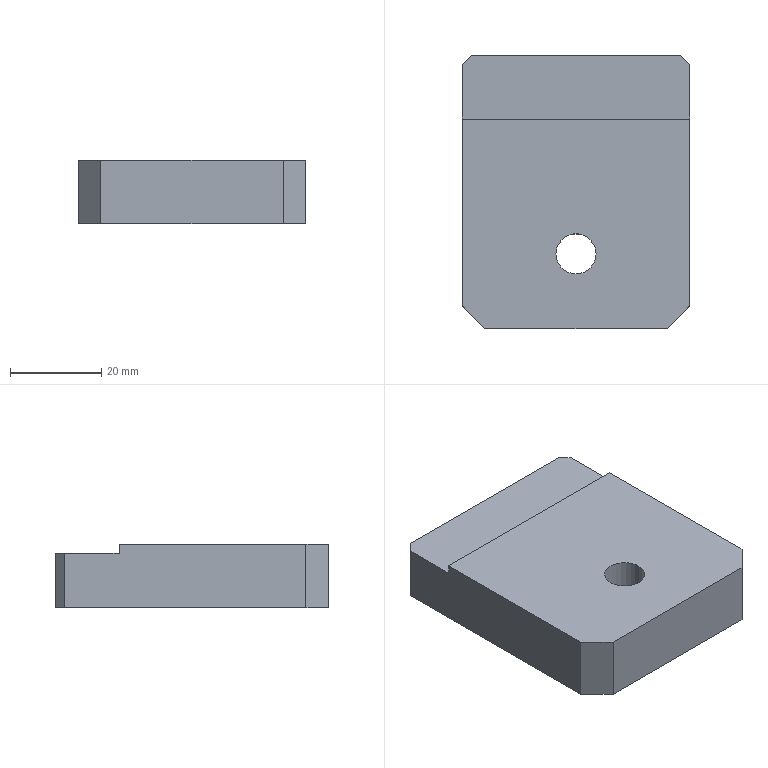Part | STEP file | 2012-06-08-03 | 1 solid | 14 faces | box 50 x 60 x 14 mm | volume 39351 mm3 | plane 12 | cylinder 2 | commonest cylinder face diameters 8.8 x2
STEP:
#1=CARTESIAN_POINT('',(0.,0.,0.));
#2=DIRECTION('',(0.,0.,1.));
#3=DIRECTION('',(1.,0.,0.));
#4=AXIS2_PLACEMENT_3D('',#1,#2,#3);
#5=CARTESIAN_POINT('',(-4.4,-13.59,14.));
#6=VERTEX_POINT('',#5);
#7=CARTESIAN_POINT('',(-4.4,-13.59,0.));
#8=VERTEX_POINT('',#7);
#9=CARTESIAN_POINT('',(-4.4,-13.59,0.));
#10=DIRECTION('',(0.,0.,-1.));
#11=VECTOR('',#10,1.);
#12=LINE('',#9,#11);
#13=CARTESIAN_POINT('',(0.,-13.59,0.));
#14=DIRECTION('',(0.,0.,-1.));
#15=DIRECTION('',(-1.,0.,0.));
#16=AXIS2_PLACEMENT_3D('',#13,#14,#15);
#17=CYLINDRICAL_SURFACE('',#16,4.4);
#18=CARTESIAN_POINT('',(6.283,0.));
#19=DIRECTION('',(0.,1.));
#20=VECTOR('',#19,1.);
#21=LINE('',#18,#20);
#22=(GEOMETRIC_REPRESENTATION_CONTEXT(2)PARAMETRIC_REPRESENTATION_CONTEXT()REPRESENTATION_CONTEXT('',''));
#23=DEFINITIONAL_REPRESENTATION('',(#21),#22);
#24=PCURVE('',#17,#23);
#25=CARTESIAN_POINT('',(0.,-13.59,0.));
#26=DIRECTION('',(0.,0.,-1.));
#27=DIRECTION('',(-1.,0.,0.));
#28=AXIS2_PLACEMENT_3D('',#25,#26,#27);
#29=CYLINDRICAL_SURFACE('',#28,4.4);
#30=CARTESIAN_POINT('',(0.,0.));
#31=DIRECTION('',(0.,1.));
#32=VECTOR('',#31,1.);
#33=LINE('',#30,#32);
#34=(GEOMETRIC_REPRESENTATION_CONTEXT(2)PARAMETRIC_REPRESENTATION_CONTEXT()REPRESENTATION_CONTEXT('',''));
#35=DEFINITIONAL_REPRESENTATION('',(#33),#34);
#36=PCURVE('',#29,#35);
#37=SURFACE_CURVE('',#12,(#24,#36),.PCURVE_S1.);
#38=EDGE_CURVE('',#6,#8,#37,.T.);
#39=ORIENTED_EDGE('',*,*,#38,.T.);
#40=CARTESIAN_POINT('',(4.4,-13.59,0.));
#41=VERTEX_POINT('',#40);
#42=CARTESIAN_POINT('',(0.,-13.59,0.));
#43=DIRECTION('',(0.,0.,-1.));
#44=DIRECTION('',(-1.,0.,0.));
#45=AXIS2_PLACEMENT_3D('',#42,#43,#44);
#46=CIRCLE('',#45,4.4);
#47=CARTESIAN_POINT('',(0.,0.));
#48=DIRECTION('',(1.,0.));
#49=VECTOR('',#48,1.);
#50=LINE('',#47,#49);
#51=(GEOMETRIC_REPRESENTATION_CONTEXT(2)PARAMETRIC_REPRESENTATION_CONTEXT()REPRESENTATION_CONTEXT('',''));
#52=DEFINITIONAL_REPRESENTATION('',(#50),#51);
#53=PCURVE('',#17,#52);
#54=CARTESIAN_POINT('',(25.,-30.,0.));
#55=DIRECTION('',(0.,0.,1.));
#56=DIRECTION('',(1.,0.,0.));
#57=AXIS2_PLACEMENT_3D('',#54,#55,#56);
#58=PLANE('',#57);
#59=CARTESIAN_POINT('',(-29.4,16.41));
#60=CARTESIAN_POINT('',(-29.4,24.031));
#61=CARTESIAN_POINT('',(-22.8,20.221));
#62=CARTESIAN_POINT('',(-16.2,16.41));
#63=CARTESIAN_POINT('',(-22.8,12.599));
#64=CARTESIAN_POINT('',(-29.4,8.789));
#65=CARTESIAN_POINT('',(-29.4,16.41));
#66=(BOUNDED_CURVE()B_SPLINE_CURVE(2,(#59,#60,#61,#62,#63,#64,#65),.UNSPECIFIED.,.T.,.F.)B_SPLINE_CURVE_WITH_KNOTS((1,2,2,2,2,1),(-2.094,0.,2.094,4.189,6.283,8.378),.UNSPECIFIED.)CURVE()GEOMETRIC_REPRESENTATION_ITEM()RATIONAL_B_SPLINE_CURVE((1.,0.5,1.,0.5,1.,0.5,1.))REPRESENTATION_ITEM(''));
#67=(GEOMETRIC_REPRESENTATION_CONTEXT(2)PARAMETRIC_REPRESENTATION_CONTEXT()REPRESENTATION_CONTEXT('',''));
#68=DEFINITIONAL_REPRESENTATION('',(#66),#67);
#69=PCURVE('',#58,#68);
#70=SURFACE_CURVE('',#46,(#53,#69),.PCURVE_S1.);
#71=EDGE_CURVE('',#41,#8,#70,.T.);
#72=ORIENTED_EDGE('',*,*,#71,.F.);
#73=CARTESIAN_POINT('',(4.4,-13.59,14.));
#74=VERTEX_POINT('',#73);
#75=CARTESIAN_POINT('',(4.4,-13.59,0.));
#76=DIRECTION('',(0.,0.,-1.));
#77=VECTOR('',#76,1.);
#78=LINE('',#75,#77);
#79=CARTESIAN_POINT('',(3.142,0.));
#80=DIRECTION('',(0.,1.));
#81=VECTOR('',#80,1.);
#82=LINE('',#79,#81);
#83=(GEOMETRIC_REPRESENTATION_CONTEXT(2)PARAMETRIC_REPRESENTATION_CONTEXT()REPRESENTATION_CONTEXT('',''));
#84=DEFINITIONAL_REPRESENTATION('',(#82),#83);
#85=PCURVE('',#17,#84);
#86=CARTESIAN_POINT('',(3.142,0.));
#87=DIRECTION('',(0.,1.));
#88=VECTOR('',#87,1.);
#89=LINE('',#86,#88);
#90=(GEOMETRIC_REPRESENTATION_CONTEXT(2)PARAMETRIC_REPRESENTATION_CONTEXT()REPRESENTATION_CONTEXT('',''));
#91=DEFINITIONAL_REPRESENTATION('',(#89),#90);
#92=PCURVE('',#29,#91);
#93=SURFACE_CURVE('',#78,(#85,#92),.PCURVE_S1.);
#94=EDGE_CURVE('',#74,#41,#93,.T.);
#95=ORIENTED_EDGE('',*,*,#94,.F.);
#96=CARTESIAN_POINT('',(0.,-13.59,14.));
#97=DIRECTION('',(0.,0.,1.));
#98=DIRECTION('',(1.,0.,0.));
#99=AXIS2_PLACEMENT_3D('',#96,#97,#98);
#100=CIRCLE('',#99,4.4);
#101=CARTESIAN_POINT('',(9.425,-14.));
#102=DIRECTION('',(-1.,0.));
#103=VECTOR('',#102,1.);
#104=LINE('',#101,#103);
#105=(GEOMETRIC_REPRESENTATION_CONTEXT(2)PARAMETRIC_REPRESENTATION_CONTEXT()REPRESENTATION_CONTEXT('',''));
#106=DEFINITIONAL_REPRESENTATION('',(#104),#105);
#107=PCURVE('',#17,#106);
#108=CARTESIAN_POINT('',(25.,-30.,14.));
#109=DIRECTION('',(0.,0.,1.));
#110=DIRECTION('',(1.,0.,0.));
#111=AXIS2_PLACEMENT_3D('',#108,#109,#110);
#112=PLANE('',#111);
#113=CARTESIAN_POINT('',(-25.,16.41));
#114=DIRECTION('',(1.,0.));
#115=AXIS2_PLACEMENT_2D('',#113,#114);
#116=CIRCLE('',#115,4.4);
#117=(GEOMETRIC_REPRESENTATION_CONTEXT(2)PARAMETRIC_REPRESENTATION_CONTEXT()REPRESENTATION_CONTEXT('',''));
#118=DEFINITIONAL_REPRESENTATION('',(#116),#117);
#119=PCURVE('',#112,#118);
#120=SURFACE_CURVE('',#100,(#107,#119),.PCURVE_S1.);
#121=EDGE_CURVE('',#6,#74,#120,.T.);
#122=ORIENTED_EDGE('',*,*,#121,.F.);
#123=EDGE_LOOP('',(#39,#72,#95,#122));
#124=FACE_BOUND('',#123,.F.);
#125=ADVANCED_FACE('',(#124),#17,.F.);
#126=CARTESIAN_POINT('',(23.,30.,12.));
#127=VERTEX_POINT('',#126);
#128=CARTESIAN_POINT('',(-23.,30.,12.));
#129=VERTEX_POINT('',#128);
#130=CARTESIAN_POINT('',(-25.,30.,12.));
#131=DIRECTION('',(-1.,0.,0.));
#132=VECTOR('',#131,1.);
#133=LINE('',#130,#132);
#134=CARTESIAN_POINT('',(-25.,30.,14.));
#135=DIRECTION('',(0.,-1.,0.));
#136=DIRECTION('',(0.,0.,-1.));
#137=AXIS2_PLACEMENT_3D('',#134,#135,#136);
#138=PLANE('',#137);
#139=CARTESIAN_POINT('',(2.,0.));
#140=DIRECTION('',(0.,-1.));
#141=VECTOR('',#140,1.);
#142=LINE('',#139,#141);
#143=(GEOMETRIC_REPRESENTATION_CONTEXT(2)PARAMETRIC_REPRESENTATION_CONTEXT()REPRESENTATION_CONTEXT('',''));
#144=DEFINITIONAL_REPRESENTATION('',(#142),#143);
#145=PCURVE('',#138,#144);
#146=CARTESIAN_POINT('',(-25.,16.,12.));
#147=DIRECTION('',(0.,0.,1.));
#148=DIRECTION('',(1.,0.,0.));
#149=AXIS2_PLACEMENT_3D('',#146,#147,#148);
#150=PLANE('',#149);
#151=CARTESIAN_POINT('',(0.,14.));
#152=DIRECTION('',(-1.,0.));
#153=VECTOR('',#152,1.);
#154=LINE('',#151,#153);
#155=(GEOMETRIC_REPRESENTATION_CONTEXT(2)PARAMETRIC_REPRESENTATION_CONTEXT()REPRESENTATION_CONTEXT('',''));
#156=DEFINITIONAL_REPRESENTATION('',(#154),#155);
#157=PCURVE('',#150,#156);
#158=SURFACE_CURVE('',#133,(#145,#157),.PCURVE_S1.);
#159=EDGE_CURVE('',#127,#129,#158,.T.);
#160=ORIENTED_EDGE('',*,*,#159,.F.);
#161=CARTESIAN_POINT('',(23.,30.,0.));
#162=VERTEX_POINT('',#161);
#163=CARTESIAN_POINT('',(23.,30.,14.));
#164=DIRECTION('',(0.,0.,-1.));
#165=VECTOR('',#164,1.);
#166=LINE('',#163,#165);
#167=CARTESIAN_POINT('',(0.,48.));
#168=DIRECTION('',(1.,0.));
#169=VECTOR('',#168,1.);
#170=LINE('',#167,#169);
#171=(GEOMETRIC_REPRESENTATION_CONTEXT(2)PARAMETRIC_REPRESENTATION_CONTEXT()REPRESENTATION_CONTEXT('',''));
#172=DEFINITIONAL_REPRESENTATION('',(#170),#171);
#173=PCURVE('',#138,#172);
#174=CARTESIAN_POINT('',(23.,30.,14.));
#175=DIRECTION('',(-0.7071,-0.7071,0.));
#176=DIRECTION('',(0.7071,-0.7071,0.));
#177=AXIS2_PLACEMENT_3D('',#174,#175,#176);
#178=PLANE('',#177);
#179=CARTESIAN_POINT('',(0.,0.));
#180=DIRECTION('',(0.,-1.));
#181=VECTOR('',#180,1.);
#182=LINE('',#179,#181);
#183=(GEOMETRIC_REPRESENTATION_CONTEXT(2)PARAMETRIC_REPRESENTATION_CONTEXT()REPRESENTATION_CONTEXT('',''));
#184=DEFINITIONAL_REPRESENTATION('',(#182),#183);
#185=PCURVE('',#178,#184);
#186=SURFACE_CURVE('',#166,(#173,#185),.PCURVE_S1.);
#187=EDGE_CURVE('',#127,#162,#186,.T.);
#188=ORIENTED_EDGE('',*,*,#187,.T.);
#189=CARTESIAN_POINT('',(-23.,30.,0.));
#190=VERTEX_POINT('',#189);
#191=CARTESIAN_POINT('',(-25.,30.,0.));
#192=DIRECTION('',(-1.,0.,0.));
#193=VECTOR('',#192,1.);
#194=LINE('',#191,#193);
#195=CARTESIAN_POINT('',(14.,0.));
#196=DIRECTION('',(0.,-1.));
#197=VECTOR('',#196,1.);
#198=LINE('',#195,#197);
#199=(GEOMETRIC_REPRESENTATION_CONTEXT(2)PARAMETRIC_REPRESENTATION_CONTEXT()REPRESENTATION_CONTEXT('',''));
#200=DEFINITIONAL_REPRESENTATION('',(#198),#199);
#201=PCURVE('',#138,#200);
#202=CARTESIAN_POINT('',(-50.,60.));
#203=DIRECTION('',(-1.,0.));
#204=VECTOR('',#203,1.);
#205=LINE('',#202,#204);
#206=(GEOMETRIC_REPRESENTATION_CONTEXT(2)PARAMETRIC_REPRESENTATION_CONTEXT()REPRESENTATION_CONTEXT('',''));
#207=DEFINITIONAL_REPRESENTATION('',(#205),#206);
#208=PCURVE('',#58,#207);
#209=SURFACE_CURVE('',#194,(#201,#208),.PCURVE_S1.);
#210=EDGE_CURVE('',#162,#190,#209,.T.);
#211=ORIENTED_EDGE('',*,*,#210,.T.);
#212=CARTESIAN_POINT('',(-23.,30.,14.));
#213=DIRECTION('',(0.,0.,1.));
#214=VECTOR('',#213,1.);
#215=LINE('',#212,#214);
#216=CARTESIAN_POINT('',(0.,2.));
#217=DIRECTION('',(-1.,0.));
#218=VECTOR('',#217,1.);
#219=LINE('',#216,#218);
#220=(GEOMETRIC_REPRESENTATION_CONTEXT(2)PARAMETRIC_REPRESENTATION_CONTEXT()REPRESENTATION_CONTEXT('',''));
#221=DEFINITIONAL_REPRESENTATION('',(#219),#220);
#222=PCURVE('',#138,#221);
#223=CARTESIAN_POINT('',(-25.,28.,14.));
#224=DIRECTION('',(0.7071,-0.7071,0.));
#225=DIRECTION('',(0.7071,0.7071,0.));
#226=AXIS2_PLACEMENT_3D('',#223,#224,#225);
#227=PLANE('',#226);
#228=CARTESIAN_POINT('',(2.828,0.));
#229=DIRECTION('',(0.,1.));
#230=VECTOR('',#229,1.);
#231=LINE('',#228,#230);
#232=(GEOMETRIC_REPRESENTATION_CONTEXT(2)PARAMETRIC_REPRESENTATION_CONTEXT()REPRESENTATION_CONTEXT('',''));
#233=DEFINITIONAL_REPRESENTATION('',(#231),#232);
#234=PCURVE('',#227,#233);
#235=SURFACE_CURVE('',#215,(#222,#234),.PCURVE_S1.);
#236=EDGE_CURVE('',#190,#129,#235,.T.);
#237=ORIENTED_EDGE('',*,*,#236,.T.);
#238=EDGE_LOOP('',(#160,#188,#211,#237));
#239=FACE_BOUND('',#238,.T.);
#240=ADVANCED_FACE('',(#239),#138,.F.);
#241=CARTESIAN_POINT('',(25.,-25.,0.));
#242=VERTEX_POINT('',#241);
#243=CARTESIAN_POINT('',(25.,28.,0.));
#244=VERTEX_POINT('',#243);
#245=CARTESIAN_POINT('',(25.,30.,0.));
#246=DIRECTION('',(0.,1.,0.));
#247=VECTOR('',#246,1.);
#248=LINE('',#245,#247);
#249=CARTESIAN_POINT('',(25.,30.,14.));
#250=DIRECTION('',(-1.,0.,0.));
#251=DIRECTION('',(0.,-1.,0.));
#252=AXIS2_PLACEMENT_3D('',#249,#250,#251);
#253=PLANE('',#252);
#254=CARTESIAN_POINT('',(0.,-14.));
#255=DIRECTION('',(-1.,0.));
#256=VECTOR('',#255,1.);
#257=LINE('',#254,#256);
#258=(GEOMETRIC_REPRESENTATION_CONTEXT(2)PARAMETRIC_REPRESENTATION_CONTEXT()REPRESENTATION_CONTEXT('',''));
#259=DEFINITIONAL_REPRESENTATION('',(#257),#258);
#260=PCURVE('',#253,#259);
#261=CARTESIAN_POINT('',(0.,60.));
#262=DIRECTION('',(0.,1.));
#263=VECTOR('',#262,1.);
#264=LINE('',#261,#263);
#265=(GEOMETRIC_REPRESENTATION_CONTEXT(2)PARAMETRIC_REPRESENTATION_CONTEXT()REPRESENTATION_CONTEXT('',''));
#266=DEFINITIONAL_REPRESENTATION('',(#264),#265);
#267=PCURVE('',#58,#266);
#268=SURFACE_CURVE('',#248,(#260,#267),.PCURVE_S1.);
#269=EDGE_CURVE('',#242,#244,#268,.T.);
#270=ORIENTED_EDGE('',*,*,#269,.T.);
#271=CARTESIAN_POINT('',(25.,28.,12.));
#272=VERTEX_POINT('',#271);
#273=CARTESIAN_POINT('',(25.,28.,14.));
#274=DIRECTION('',(0.,0.,1.));
#275=VECTOR('',#274,1.);
#276=LINE('',#273,#275);
#277=CARTESIAN_POINT('',(2.,0.));
#278=DIRECTION('',(0.,1.));
#279=VECTOR('',#278,1.);
#280=LINE('',#277,#279);
#281=(GEOMETRIC_REPRESENTATION_CONTEXT(2)PARAMETRIC_REPRESENTATION_CONTEXT()REPRESENTATION_CONTEXT('',''));
#282=DEFINITIONAL_REPRESENTATION('',(#280),#281);
#283=PCURVE('',#253,#282);
#284=CARTESIAN_POINT('',(2.828,0.));
#285=DIRECTION('',(0.,1.));
#286=VECTOR('',#285,1.);
#287=LINE('',#284,#286);
#288=(GEOMETRIC_REPRESENTATION_CONTEXT(2)PARAMETRIC_REPRESENTATION_CONTEXT()REPRESENTATION_CONTEXT('',''));
#289=DEFINITIONAL_REPRESENTATION('',(#287),#288);
#290=PCURVE('',#178,#289);
#291=SURFACE_CURVE('',#276,(#283,#290),.PCURVE_S1.);
#292=EDGE_CURVE('',#244,#272,#291,.T.);
#293=ORIENTED_EDGE('',*,*,#292,.T.);
#294=CARTESIAN_POINT('',(25.,16.,12.));
#295=VERTEX_POINT('',#294);
#296=CARTESIAN_POINT('',(25.,30.,12.));
#297=DIRECTION('',(0.,1.,0.));
#298=VECTOR('',#297,1.);
#299=LINE('',#296,#298);
#300=CARTESIAN_POINT('',(0.,-2.));
#301=DIRECTION('',(-1.,0.));
#302=VECTOR('',#301,1.);
#303=LINE('',#300,#302);
#304=(GEOMETRIC_REPRESENTATION_CONTEXT(2)PARAMETRIC_REPRESENTATION_CONTEXT()REPRESENTATION_CONTEXT('',''));
#305=DEFINITIONAL_REPRESENTATION('',(#303),#304);
#306=PCURVE('',#253,#305);
#307=CARTESIAN_POINT('',(50.,14.));
#308=DIRECTION('',(0.,1.));
#309=VECTOR('',#308,1.);
#310=LINE('',#307,#309);
#311=(GEOMETRIC_REPRESENTATION_CONTEXT(2)PARAMETRIC_REPRESENTATION_CONTEXT()REPRESENTATION_CONTEXT('',''));
#312=DEFINITIONAL_REPRESENTATION('',(#310),#311);
#313=PCURVE('',#150,#312);
#314=SURFACE_CURVE('',#299,(#306,#313),.PCURVE_S1.);
#315=EDGE_CURVE('',#295,#272,#314,.T.);
#316=ORIENTED_EDGE('',*,*,#315,.F.);
#317=CARTESIAN_POINT('',(25.,16.,14.));
#318=VERTEX_POINT('',#317);
#319=CARTESIAN_POINT('',(25.,16.,12.));
#320=DIRECTION('',(0.,0.,1.));
#321=VECTOR('',#320,1.);
#322=LINE('',#319,#321);
#323=CARTESIAN_POINT('',(14.,-2.));
#324=DIRECTION('',(0.,1.));
#325=VECTOR('',#324,1.);
#326=LINE('',#323,#325);
#327=(GEOMETRIC_REPRESENTATION_CONTEXT(2)PARAMETRIC_REPRESENTATION_CONTEXT()REPRESENTATION_CONTEXT('',''));
#328=DEFINITIONAL_REPRESENTATION('',(#326),#327);
#329=PCURVE('',#253,#328);
#330=CARTESIAN_POINT('',(-25.,16.,12.));
#331=DIRECTION('',(0.,-1.,0.));
#332=DIRECTION('',(0.,0.,-1.));
#333=AXIS2_PLACEMENT_3D('',#330,#331,#332);
#334=PLANE('',#333);
#335=CARTESIAN_POINT('',(0.,50.));
#336=DIRECTION('',(-1.,0.));
#337=VECTOR('',#336,1.);
#338=LINE('',#335,#337);
#339=(GEOMETRIC_REPRESENTATION_CONTEXT(2)PARAMETRIC_REPRESENTATION_CONTEXT()REPRESENTATION_CONTEXT('',''));
#340=DEFINITIONAL_REPRESENTATION('',(#338),#339);
#341=PCURVE('',#334,#340);
#342=SURFACE_CURVE('',#322,(#329,#341),.PCURVE_S1.);
#343=EDGE_CURVE('',#295,#318,#342,.T.);
#344=ORIENTED_EDGE('',*,*,#343,.T.);
#345=CARTESIAN_POINT('',(25.,-25.,14.));
#346=VERTEX_POINT('',#345);
#347=CARTESIAN_POINT('',(25.,30.,14.));
#348=DIRECTION('',(0.,1.,0.));
#349=VECTOR('',#348,1.);
#350=LINE('',#347,#349);
#351=CARTESIAN_POINT('',(0.,0.));
#352=DIRECTION('',(-1.,0.));
#353=VECTOR('',#352,1.);
#354=LINE('',#351,#353);
#355=(GEOMETRIC_REPRESENTATION_CONTEXT(2)PARAMETRIC_REPRESENTATION_CONTEXT()REPRESENTATION_CONTEXT('',''));
#356=DEFINITIONAL_REPRESENTATION('',(#354),#355);
#357=PCURVE('',#253,#356);
#358=CARTESIAN_POINT('',(0.,60.));
#359=DIRECTION('',(0.,1.));
#360=VECTOR('',#359,1.);
#361=LINE('',#358,#360);
#362=(GEOMETRIC_REPRESENTATION_CONTEXT(2)PARAMETRIC_REPRESENTATION_CONTEXT()REPRESENTATION_CONTEXT('',''));
#363=DEFINITIONAL_REPRESENTATION('',(#361),#362);
#364=PCURVE('',#112,#363);
#365=SURFACE_CURVE('',#350,(#357,#364),.PCURVE_S1.);
#366=EDGE_CURVE('',#346,#318,#365,.T.);
#367=ORIENTED_EDGE('',*,*,#366,.F.);
#368=CARTESIAN_POINT('',(25.,-25.,14.));
#369=DIRECTION('',(0.,0.,-1.));
#370=VECTOR('',#369,1.);
#371=LINE('',#368,#370);
#372=CARTESIAN_POINT('',(55.,0.));
#373=DIRECTION('',(0.,-1.));
#374=VECTOR('',#373,1.);
#375=LINE('',#372,#374);
#376=(GEOMETRIC_REPRESENTATION_CONTEXT(2)PARAMETRIC_REPRESENTATION_CONTEXT()REPRESENTATION_CONTEXT('',''));
#377=DEFINITIONAL_REPRESENTATION('',(#375),#376);
#378=PCURVE('',#253,#377);
#379=CARTESIAN_POINT('',(25.,-25.,14.));
#380=DIRECTION('',(-0.7071,0.7071,0.));
#381=DIRECTION('',(-0.7071,-0.7071,0.));
#382=AXIS2_PLACEMENT_3D('',#379,#380,#381);
#383=PLANE('',#382);
#384=CARTESIAN_POINT('',(0.,0.));
#385=DIRECTION('',(0.,-1.));
#386=VECTOR('',#385,1.);
#387=LINE('',#384,#386);
#388=(GEOMETRIC_REPRESENTATION_CONTEXT(2)PARAMETRIC_REPRESENTATION_CONTEXT()REPRESENTATION_CONTEXT('',''));
#389=DEFINITIONAL_REPRESENTATION('',(#387),#388);
#390=PCURVE('',#383,#389);
#391=SURFACE_CURVE('',#371,(#378,#390),.PCURVE_S1.);
#392=EDGE_CURVE('',#346,#242,#391,.T.);
#393=ORIENTED_EDGE('',*,*,#392,.T.);
#394=EDGE_LOOP('',(#270,#293,#316,#344,#367,#393));
#395=FACE_BOUND('',#394,.T.);
#396=ADVANCED_FACE('',(#395),#253,.F.);
#397=CARTESIAN_POINT('',(-25.,28.,12.));
#398=VERTEX_POINT('',#397);
#399=CARTESIAN_POINT('',(-25.,16.,12.));
#400=VERTEX_POINT('',#399);
#401=CARTESIAN_POINT('',(-25.,30.,12.));
#402=DIRECTION('',(0.,-1.,0.));
#403=VECTOR('',#402,1.);
#404=LINE('',#401,#403);
#405=CARTESIAN_POINT('',(-25.,30.,14.));
#406=DIRECTION('',(1.,0.,0.));
#407=DIRECTION('',(0.,1.,0.));
#408=AXIS2_PLACEMENT_3D('',#405,#406,#407);
#409=PLANE('',#408);
#410=CARTESIAN_POINT('',(0.,-2.));
#411=DIRECTION('',(-1.,0.));
#412=VECTOR('',#411,1.);
#413=LINE('',#410,#412);
#414=(GEOMETRIC_REPRESENTATION_CONTEXT(2)PARAMETRIC_REPRESENTATION_CONTEXT()REPRESENTATION_CONTEXT('',''));
#415=DEFINITIONAL_REPRESENTATION('',(#413),#414);
#416=PCURVE('',#409,#415);
#417=CARTESIAN_POINT('',(0.,14.));
#418=DIRECTION('',(0.,-1.));
#419=VECTOR('',#418,1.);
#420=LINE('',#417,#419);
#421=(GEOMETRIC_REPRESENTATION_CONTEXT(2)PARAMETRIC_REPRESENTATION_CONTEXT()REPRESENTATION_CONTEXT('',''));
#422=DEFINITIONAL_REPRESENTATION('',(#420),#421);
#423=PCURVE('',#150,#422);
#424=SURFACE_CURVE('',#404,(#416,#423),.PCURVE_S1.);
#425=EDGE_CURVE('',#398,#400,#424,.T.);
#426=ORIENTED_EDGE('',*,*,#425,.F.);
#427=CARTESIAN_POINT('',(-25.,28.,0.));
#428=VERTEX_POINT('',#427);
#429=CARTESIAN_POINT('',(-25.,28.,14.));
#430=DIRECTION('',(0.,0.,-1.));
#431=VECTOR('',#430,1.);
#432=LINE('',#429,#431);
#433=CARTESIAN_POINT('',(-2.,0.));
#434=DIRECTION('',(0.,-1.));
#435=VECTOR('',#434,1.);
#436=LINE('',#433,#435);
#437=(GEOMETRIC_REPRESENTATION_CONTEXT(2)PARAMETRIC_REPRESENTATION_CONTEXT()REPRESENTATION_CONTEXT('',''));
#438=DEFINITIONAL_REPRESENTATION('',(#436),#437);
#439=PCURVE('',#409,#438);
#440=CARTESIAN_POINT('',(0.,0.));
#441=DIRECTION('',(0.,-1.));
#442=VECTOR('',#441,1.);
#443=LINE('',#440,#442);
#444=(GEOMETRIC_REPRESENTATION_CONTEXT(2)PARAMETRIC_REPRESENTATION_CONTEXT()REPRESENTATION_CONTEXT('',''));
#445=DEFINITIONAL_REPRESENTATION('',(#443),#444);
#446=PCURVE('',#227,#445);
#447=SURFACE_CURVE('',#432,(#439,#446),.PCURVE_S1.);
#448=EDGE_CURVE('',#398,#428,#447,.T.);
#449=ORIENTED_EDGE('',*,*,#448,.T.);
#450=CARTESIAN_POINT('',(-25.,-25.,0.));
#451=VERTEX_POINT('',#450);
#452=CARTESIAN_POINT('',(-25.,30.,0.));
#453=DIRECTION('',(0.,-1.,0.));
#454=VECTOR('',#453,1.);
#455=LINE('',#452,#454);
#456=CARTESIAN_POINT('',(0.,-14.));
#457=DIRECTION('',(-1.,0.));
#458=VECTOR('',#457,1.);
#459=LINE('',#456,#458);
#460=(GEOMETRIC_REPRESENTATION_CONTEXT(2)PARAMETRIC_REPRESENTATION_CONTEXT()REPRESENTATION_CONTEXT('',''));
#461=DEFINITIONAL_REPRESENTATION('',(#459),#460);
#462=PCURVE('',#409,#461);
#463=CARTESIAN_POINT('',(-50.,60.));
#464=DIRECTION('',(0.,-1.));
#465=VECTOR('',#464,1.);
#466=LINE('',#463,#465);
#467=(GEOMETRIC_REPRESENTATION_CONTEXT(2)PARAMETRIC_REPRESENTATION_CONTEXT()REPRESENTATION_CONTEXT('',''));
#468=DEFINITIONAL_REPRESENTATION('',(#466),#467);
#469=PCURVE('',#58,#468);
#470=SURFACE_CURVE('',#455,(#462,#469),.PCURVE_S1.);
#471=EDGE_CURVE('',#428,#451,#470,.T.);
#472=ORIENTED_EDGE('',*,*,#471,.T.);
#473=CARTESIAN_POINT('',(-25.,-25.,14.));
#474=VERTEX_POINT('',#473);
#475=CARTESIAN_POINT('',(-25.,-25.,14.));
#476=DIRECTION('',(0.,0.,1.));
#477=VECTOR('',#476,1.);
#478=LINE('',#475,#477);
#479=CARTESIAN_POINT('',(-55.,0.));
#480=DIRECTION('',(0.,1.));
#481=VECTOR('',#480,1.);
#482=LINE('',#479,#481);
#483=(GEOMETRIC_REPRESENTATION_CONTEXT(2)PARAMETRIC_REPRESENTATION_CONTEXT()REPRESENTATION_CONTEXT('',''));
#484=DEFINITIONAL_REPRESENTATION('',(#482),#483);
#485=PCURVE('',#409,#484);
#486=CARTESIAN_POINT('',(-20.,-30.,14.));
#487=DIRECTION('',(0.7071,0.7071,0.));
#488=DIRECTION('',(-0.7071,0.7071,0.));
#489=AXIS2_PLACEMENT_3D('',#486,#487,#488);
#490=PLANE('',#489);
#491=CARTESIAN_POINT('',(7.071,0.));
#492=DIRECTION('',(0.,1.));
#493=VECTOR('',#492,1.);
#494=LINE('',#491,#493);
#495=(GEOMETRIC_REPRESENTATION_CONTEXT(2)PARAMETRIC_REPRESENTATION_CONTEXT()REPRESENTATION_CONTEXT('',''));
#496=DEFINITIONAL_REPRESENTATION('',(#494),#495);
#497=PCURVE('',#490,#496);
#498=SURFACE_CURVE('',#478,(#485,#497),.PCURVE_S1.);
#499=EDGE_CURVE('',#451,#474,#498,.T.);
#500=ORIENTED_EDGE('',*,*,#499,.T.);
#501=CARTESIAN_POINT('',(-25.,16.,14.));
#502=VERTEX_POINT('',#501);
#503=CARTESIAN_POINT('',(-25.,30.,14.));
#504=DIRECTION('',(0.,-1.,0.));
#505=VECTOR('',#504,1.);
#506=LINE('',#503,#505);
#507=CARTESIAN_POINT('',(0.,0.));
#508=DIRECTION('',(-1.,0.));
#509=VECTOR('',#508,1.);
#510=LINE('',#507,#509);
#511=(GEOMETRIC_REPRESENTATION_CONTEXT(2)PARAMETRIC_REPRESENTATION_CONTEXT()REPRESENTATION_CONTEXT('',''));
#512=DEFINITIONAL_REPRESENTATION('',(#510),#511);
#513=PCURVE('',#409,#512);
#514=CARTESIAN_POINT('',(-50.,60.));
#515=DIRECTION('',(0.,-1.));
#516=VECTOR('',#515,1.);
#517=LINE('',#514,#516);
#518=(GEOMETRIC_REPRESENTATION_CONTEXT(2)PARAMETRIC_REPRESENTATION_CONTEXT()REPRESENTATION_CONTEXT('',''));
#519=DEFINITIONAL_REPRESENTATION('',(#517),#518);
#520=PCURVE('',#112,#519);
#521=SURFACE_CURVE('',#506,(#513,#520),.PCURVE_S1.);
#522=EDGE_CURVE('',#502,#474,#521,.T.);
#523=ORIENTED_EDGE('',*,*,#522,.F.);
#524=CARTESIAN_POINT('',(-25.,16.,12.));
#525=DIRECTION('',(0.,0.,1.));
#526=VECTOR('',#525,1.);
#527=LINE('',#524,#526);
#528=CARTESIAN_POINT('',(-14.,-2.));
#529=DIRECTION('',(0.,1.));
#530=VECTOR('',#529,1.);
#531=LINE('',#528,#530);
#532=(GEOMETRIC_REPRESENTATION_CONTEXT(2)PARAMETRIC_REPRESENTATION_CONTEXT()REPRESENTATION_CONTEXT('',''));
#533=DEFINITIONAL_REPRESENTATION('',(#531),#532);
#534=PCURVE('',#409,#533);
#535=CARTESIAN_POINT('',(0.,0.));
#536=DIRECTION('',(-1.,0.));
#537=VECTOR('',#536,1.);
#538=LINE('',#535,#537);
#539=(GEOMETRIC_REPRESENTATION_CONTEXT(2)PARAMETRIC_REPRESENTATION_CONTEXT()REPRESENTATION_CONTEXT('',''));
#540=DEFINITIONAL_REPRESENTATION('',(#538),#539);
#541=PCURVE('',#334,#540);
#542=SURFACE_CURVE('',#527,(#534,#541),.PCURVE_S1.);
#543=EDGE_CURVE('',#400,#502,#542,.T.);
#544=ORIENTED_EDGE('',*,*,#543,.F.);
#545=EDGE_LOOP('',(#426,#449,#472,#500,#523,#544));
#546=FACE_BOUND('',#545,.T.);
#547=ADVANCED_FACE('',(#546),#409,.F.);
#548=CARTESIAN_POINT('',(-20.,-30.,0.));
#549=VERTEX_POINT('',#548);
#550=CARTESIAN_POINT('',(20.,-30.,0.));
#551=VERTEX_POINT('',#550);
#552=CARTESIAN_POINT('',(-25.,-30.,0.));
#553=DIRECTION('',(1.,0.,0.));
#554=VECTOR('',#553,1.);
#555=LINE('',#552,#554);
#556=CARTESIAN_POINT('',(-25.,-30.,14.));
#557=DIRECTION('',(0.,1.,0.));
#558=DIRECTION('',(0.,0.,1.));
#559=AXIS2_PLACEMENT_3D('',#556,#557,#558);
#560=PLANE('',#559);
#561=CARTESIAN_POINT('',(-14.,0.));
#562=DIRECTION('',(0.,1.));
#563=VECTOR('',#562,1.);
#564=LINE('',#561,#563);
#565=(GEOMETRIC_REPRESENTATION_CONTEXT(2)PARAMETRIC_REPRESENTATION_CONTEXT()REPRESENTATION_CONTEXT('',''));
#566=DEFINITIONAL_REPRESENTATION('',(#564),#565);
#567=PCURVE('',#560,#566);
#568=CARTESIAN_POINT('',(-50.,0.));
#569=DIRECTION('',(1.,0.));
#570=VECTOR('',#569,1.);
#571=LINE('',#568,#570);
#572=(GEOMETRIC_REPRESENTATION_CONTEXT(2)PARAMETRIC_REPRESENTATION_CONTEXT()REPRESENTATION_CONTEXT('',''));
#573=DEFINITIONAL_REPRESENTATION('',(#571),#572);
#574=PCURVE('',#58,#573);
#575=SURFACE_CURVE('',#555,(#567,#574),.PCURVE_S1.);
#576=EDGE_CURVE('',#549,#551,#575,.T.);
#577=ORIENTED_EDGE('',*,*,#576,.T.);
#578=CARTESIAN_POINT('',(20.,-30.,14.));
#579=VERTEX_POINT('',#578);
#580=CARTESIAN_POINT('',(20.,-30.,14.));
#581=DIRECTION('',(0.,0.,1.));
#582=VECTOR('',#581,1.);
#583=LINE('',#580,#582);
#584=CARTESIAN_POINT('',(0.,45.));
#585=DIRECTION('',(1.,0.));
#586=VECTOR('',#585,1.);
#587=LINE('',#584,#586);
#588=(GEOMETRIC_REPRESENTATION_CONTEXT(2)PARAMETRIC_REPRESENTATION_CONTEXT()REPRESENTATION_CONTEXT('',''));
#589=DEFINITIONAL_REPRESENTATION('',(#587),#588);
#590=PCURVE('',#560,#589);
#591=CARTESIAN_POINT('',(7.071,0.));
#592=DIRECTION('',(0.,1.));
#593=VECTOR('',#592,1.);
#594=LINE('',#591,#593);
#595=(GEOMETRIC_REPRESENTATION_CONTEXT(2)PARAMETRIC_REPRESENTATION_CONTEXT()REPRESENTATION_CONTEXT('',''));
#596=DEFINITIONAL_REPRESENTATION('',(#594),#595);
#597=PCURVE('',#383,#596);
#598=SURFACE_CURVE('',#583,(#590,#597),.PCURVE_S1.);
#599=EDGE_CURVE('',#551,#579,#598,.T.);
#600=ORIENTED_EDGE('',*,*,#599,.T.);
#601=CARTESIAN_POINT('',(-20.,-30.,14.));
#602=VERTEX_POINT('',#601);
#603=CARTESIAN_POINT('',(-25.,-30.,14.));
#604=DIRECTION('',(1.,0.,0.));
#605=VECTOR('',#604,1.);
#606=LINE('',#603,#605);
#607=CARTESIAN_POINT('',(0.,0.));
#608=DIRECTION('',(0.,1.));
#609=VECTOR('',#608,1.);
#610=LINE('',#607,#609);
#611=(GEOMETRIC_REPRESENTATION_CONTEXT(2)PARAMETRIC_REPRESENTATION_CONTEXT()REPRESENTATION_CONTEXT('',''));
#612=DEFINITIONAL_REPRESENTATION('',(#610),#611);
#613=PCURVE('',#560,#612);
#614=CARTESIAN_POINT('',(-50.,0.));
#615=DIRECTION('',(1.,0.));
#616=VECTOR('',#615,1.);
#617=LINE('',#614,#616);
#618=(GEOMETRIC_REPRESENTATION_CONTEXT(2)PARAMETRIC_REPRESENTATION_CONTEXT()REPRESENTATION_CONTEXT('',''));
#619=DEFINITIONAL_REPRESENTATION('',(#617),#618);
#620=PCURVE('',#112,#619);
#621=SURFACE_CURVE('',#606,(#613,#620),.PCURVE_S1.);
#622=EDGE_CURVE('',#602,#579,#621,.T.);
#623=ORIENTED_EDGE('',*,*,#622,.F.);
#624=CARTESIAN_POINT('',(-20.,-30.,14.));
#625=DIRECTION('',(0.,0.,-1.));
#626=VECTOR('',#625,1.);
#627=LINE('',#624,#626);
#628=CARTESIAN_POINT('',(0.,5.));
#629=DIRECTION('',(-1.,0.));
#630=VECTOR('',#629,1.);
#631=LINE('',#628,#630);
#632=(GEOMETRIC_REPRESENTATION_CONTEXT(2)PARAMETRIC_REPRESENTATION_CONTEXT()REPRESENTATION_CONTEXT('',''));
#633=DEFINITIONAL_REPRESENTATION('',(#631),#632);
#634=PCURVE('',#560,#633);
#635=CARTESIAN_POINT('',(0.,0.));
#636=DIRECTION('',(0.,-1.));
#637=VECTOR('',#636,1.);
#638=LINE('',#635,#637);
#639=(GEOMETRIC_REPRESENTATION_CONTEXT(2)PARAMETRIC_REPRESENTATION_CONTEXT()REPRESENTATION_CONTEXT('',''));
#640=DEFINITIONAL_REPRESENTATION('',(#638),#639);
#641=PCURVE('',#490,#640);
#642=SURFACE_CURVE('',#627,(#634,#641),.PCURVE_S1.);
#643=EDGE_CURVE('',#602,#549,#642,.T.);
#644=ORIENTED_EDGE('',*,*,#643,.T.);
#645=EDGE_LOOP('',(#577,#600,#623,#644));
#646=FACE_BOUND('',#645,.T.);
#647=ADVANCED_FACE('',(#646),#560,.F.);
#648=ORIENTED_EDGE('',*,*,#121,.F.);
#649=CARTESIAN_POINT('',(0.,-13.59,14.));
#650=DIRECTION('',(0.,0.,1.));
#651=DIRECTION('',(1.,0.,0.));
#652=AXIS2_PLACEMENT_3D('',#649,#650,#651);
#653=CIRCLE('',#652,4.4);
#654=CARTESIAN_POINT('',(-25.,16.41));
#655=DIRECTION('',(1.,0.));
#656=AXIS2_PLACEMENT_2D('',#654,#655);
#657=CIRCLE('',#656,4.4);
#658=(GEOMETRIC_REPRESENTATION_CONTEXT(2)PARAMETRIC_REPRESENTATION_CONTEXT()REPRESENTATION_CONTEXT('',''));
#659=DEFINITIONAL_REPRESENTATION('',(#657),#658);
#660=PCURVE('',#112,#659);
#661=CARTESIAN_POINT('',(3.142,-14.));
#662=DIRECTION('',(-1.,0.));
#663=VECTOR('',#662,1.);
#664=LINE('',#661,#663);
#665=(GEOMETRIC_REPRESENTATION_CONTEXT(2)PARAMETRIC_REPRESENTATION_CONTEXT()REPRESENTATION_CONTEXT('',''));
#666=DEFINITIONAL_REPRESENTATION('',(#664),#665);
#667=PCURVE('',#29,#666);
#668=SURFACE_CURVE('',#653,(#660,#667),.PCURVE_S1.);
#669=EDGE_CURVE('',#74,#6,#668,.T.);
#670=ORIENTED_EDGE('',*,*,#669,.F.);
#671=EDGE_LOOP('',(#648,#670));
#672=FACE_BOUND('',#671,.T.);
#673=ORIENTED_EDGE('',*,*,#622,.T.);
#674=CARTESIAN_POINT('',(22.5,-27.5,14.));
#675=DIRECTION('',(0.7071,0.7071,0.));
#676=VECTOR('',#675,1.);
#677=LINE('',#674,#676);
#678=CARTESIAN_POINT('',(-2.5,2.5));
#679=DIRECTION('',(0.7071,0.7071));
#680=VECTOR('',#679,1.);
#681=LINE('',#678,#680);
#682=(GEOMETRIC_REPRESENTATION_CONTEXT(2)PARAMETRIC_REPRESENTATION_CONTEXT()REPRESENTATION_CONTEXT('',''));
#683=DEFINITIONAL_REPRESENTATION('',(#681),#682);
#684=PCURVE('',#112,#683);
#685=CARTESIAN_POINT('',(3.536,0.));
#686=DIRECTION('',(-1.,0.));
#687=VECTOR('',#686,1.);
#688=LINE('',#685,#687);
#689=(GEOMETRIC_REPRESENTATION_CONTEXT(2)PARAMETRIC_REPRESENTATION_CONTEXT()REPRESENTATION_CONTEXT('',''));
#690=DEFINITIONAL_REPRESENTATION('',(#688),#689);
#691=PCURVE('',#383,#690);
#692=SURFACE_CURVE('',#677,(#684,#691),.PCURVE_S1.);
#693=EDGE_CURVE('',#579,#346,#692,.T.);
#694=ORIENTED_EDGE('',*,*,#693,.T.);
#695=ORIENTED_EDGE('',*,*,#366,.T.);
#696=CARTESIAN_POINT('',(-25.,16.,14.));
#697=DIRECTION('',(1.,0.,0.));
#698=VECTOR('',#697,1.);
#699=LINE('',#696,#698);
#700=CARTESIAN_POINT('',(-50.,46.));
#701=DIRECTION('',(1.,0.));
#702=VECTOR('',#701,1.);
#703=LINE('',#700,#702);
#704=(GEOMETRIC_REPRESENTATION_CONTEXT(2)PARAMETRIC_REPRESENTATION_CONTEXT()REPRESENTATION_CONTEXT('',''));
#705=DEFINITIONAL_REPRESENTATION('',(#703),#704);
#706=PCURVE('',#112,#705);
#707=CARTESIAN_POINT('',(-2.,0.));
#708=DIRECTION('',(0.,1.));
#709=VECTOR('',#708,1.);
#710=LINE('',#707,#709);
#711=(GEOMETRIC_REPRESENTATION_CONTEXT(2)PARAMETRIC_REPRESENTATION_CONTEXT()REPRESENTATION_CONTEXT('',''));
#712=DEFINITIONAL_REPRESENTATION('',(#710),#711);
#713=PCURVE('',#334,#712);
#714=SURFACE_CURVE('',#699,(#706,#713),.PCURVE_S1.);
#715=EDGE_CURVE('',#502,#318,#714,.T.);
#716=ORIENTED_EDGE('',*,*,#715,.F.);
#717=ORIENTED_EDGE('',*,*,#522,.T.);
#718=CARTESIAN_POINT('',(2.5,-52.5,14.));
#719=DIRECTION('',(0.7071,-0.7071,0.));
#720=VECTOR('',#719,1.);
#721=LINE('',#718,#720);
#722=CARTESIAN_POINT('',(-22.5,-22.5));
#723=DIRECTION('',(0.7071,-0.7071));
#724=VECTOR('',#723,1.);
#725=LINE('',#722,#724);
#726=(GEOMETRIC_REPRESENTATION_CONTEXT(2)PARAMETRIC_REPRESENTATION_CONTEXT()REPRESENTATION_CONTEXT('',''));
#727=DEFINITIONAL_REPRESENTATION('',(#725),#726);
#728=PCURVE('',#112,#727);
#729=CARTESIAN_POINT('',(-31.82,0.));
#730=DIRECTION('',(-1.,0.));
#731=VECTOR('',#730,1.);
#732=LINE('',#729,#731);
#733=(GEOMETRIC_REPRESENTATION_CONTEXT(2)PARAMETRIC_REPRESENTATION_CONTEXT()REPRESENTATION_CONTEXT('',''));
#734=DEFINITIONAL_REPRESENTATION('',(#732),#733);
#735=PCURVE('',#490,#734);
#736=SURFACE_CURVE('',#721,(#728,#735),.PCURVE_S1.);
#737=EDGE_CURVE('',#474,#602,#736,.T.);
#738=ORIENTED_EDGE('',*,*,#737,.T.);
#739=EDGE_LOOP('',(#673,#694,#695,#716,#717,#738));
#740=FACE_BOUND('',#739,.T.);
#741=ADVANCED_FACE('',(#672,#740),#112,.T.);
#742=CARTESIAN_POINT('',(0.,-13.59,0.));
#743=DIRECTION('',(0.,0.,-1.));
#744=DIRECTION('',(-1.,0.,0.));
#745=AXIS2_PLACEMENT_3D('',#742,#743,#744);
#746=CIRCLE('',#745,4.4);
#747=CARTESIAN_POINT('',(-29.4,16.41));
#748=CARTESIAN_POINT('',(-29.4,24.031));
#749=CARTESIAN_POINT('',(-22.8,20.221));
#750=CARTESIAN_POINT('',(-16.2,16.41));
#751=CARTESIAN_POINT('',(-22.8,12.599));
#752=CARTESIAN_POINT('',(-29.4,8.789));
#753=CARTESIAN_POINT('',(-29.4,16.41));
#754=(BOUNDED_CURVE()B_SPLINE_CURVE(2,(#747,#748,#749,#750,#751,#752,#753),.UNSPECIFIED.,.T.,.F.)B_SPLINE_CURVE_WITH_KNOTS((1,2,2,2,2,1),(-2.094,0.,2.094,4.189,6.283,8.378),.UNSPECIFIED.)CURVE()GEOMETRIC_REPRESENTATION_ITEM()RATIONAL_B_SPLINE_CURVE((1.,0.5,1.,0.5,1.,0.5,1.))REPRESENTATION_ITEM(''));
#755=(GEOMETRIC_REPRESENTATION_CONTEXT(2)PARAMETRIC_REPRESENTATION_CONTEXT()REPRESENTATION_CONTEXT('',''));
#756=DEFINITIONAL_REPRESENTATION('',(#754),#755);
#757=PCURVE('',#58,#756);
#758=CARTESIAN_POINT('',(0.,0.));
#759=DIRECTION('',(1.,0.));
#760=VECTOR('',#759,1.);
#761=LINE('',#758,#760);
#762=(GEOMETRIC_REPRESENTATION_CONTEXT(2)PARAMETRIC_REPRESENTATION_CONTEXT()REPRESENTATION_CONTEXT('',''));
#763=DEFINITIONAL_REPRESENTATION('',(#761),#762);
#764=PCURVE('',#29,#763);
#765=SURFACE_CURVE('',#746,(#757,#764),.PCURVE_S1.);
#766=EDGE_CURVE('',#8,#41,#765,.T.);
#767=ORIENTED_EDGE('',*,*,#766,.F.);
#768=ORIENTED_EDGE('',*,*,#71,.F.);
#769=EDGE_LOOP('',(#767,#768));
#770=FACE_BOUND('',#769,.T.);
#771=ORIENTED_EDGE('',*,*,#210,.F.);
#772=CARTESIAN_POINT('',(23.,30.,0.));
#773=DIRECTION('',(0.7071,-0.7071,0.));
#774=VECTOR('',#773,1.);
#775=LINE('',#772,#774);
#776=CARTESIAN_POINT('',(-2.,60.));
#777=DIRECTION('',(0.7071,-0.7071));
#778=VECTOR('',#777,1.);
#779=LINE('',#776,#778);
#780=(GEOMETRIC_REPRESENTATION_CONTEXT(2)PARAMETRIC_REPRESENTATION_CONTEXT()REPRESENTATION_CONTEXT('',''));
#781=DEFINITIONAL_REPRESENTATION('',(#779),#780);
#782=PCURVE('',#58,#781);
#783=CARTESIAN_POINT('',(0.,-14.));
#784=DIRECTION('',(1.,0.));
#785=VECTOR('',#784,1.);
#786=LINE('',#783,#785);
#787=(GEOMETRIC_REPRESENTATION_CONTEXT(2)PARAMETRIC_REPRESENTATION_CONTEXT()REPRESENTATION_CONTEXT('',''));
#788=DEFINITIONAL_REPRESENTATION('',(#786),#787);
#789=PCURVE('',#178,#788);
#790=SURFACE_CURVE('',#775,(#782,#789),.PCURVE_S1.);
#791=EDGE_CURVE('',#162,#244,#790,.T.);
#792=ORIENTED_EDGE('',*,*,#791,.T.);
#793=ORIENTED_EDGE('',*,*,#269,.F.);
#794=CARTESIAN_POINT('',(25.,-25.,0.));
#795=DIRECTION('',(-0.7071,-0.7071,0.));
#796=VECTOR('',#795,1.);
#797=LINE('',#794,#796);
#798=CARTESIAN_POINT('',(0.,5.));
#799=DIRECTION('',(-0.7071,-0.7071));
#800=VECTOR('',#799,1.);
#801=LINE('',#798,#800);
#802=(GEOMETRIC_REPRESENTATION_CONTEXT(2)PARAMETRIC_REPRESENTATION_CONTEXT()REPRESENTATION_CONTEXT('',''));
#803=DEFINITIONAL_REPRESENTATION('',(#801),#802);
#804=PCURVE('',#58,#803);
#805=CARTESIAN_POINT('',(0.,-14.));
#806=DIRECTION('',(1.,0.));
#807=VECTOR('',#806,1.);
#808=LINE('',#805,#807);
#809=(GEOMETRIC_REPRESENTATION_CONTEXT(2)PARAMETRIC_REPRESENTATION_CONTEXT()REPRESENTATION_CONTEXT('',''));
#810=DEFINITIONAL_REPRESENTATION('',(#808),#809);
#811=PCURVE('',#383,#810);
#812=SURFACE_CURVE('',#797,(#804,#811),.PCURVE_S1.);
#813=EDGE_CURVE('',#242,#551,#812,.T.);
#814=ORIENTED_EDGE('',*,*,#813,.T.);
#815=ORIENTED_EDGE('',*,*,#576,.F.);
#816=CARTESIAN_POINT('',(-20.,-30.,0.));
#817=DIRECTION('',(-0.7071,0.7071,0.));
#818=VECTOR('',#817,1.);
#819=LINE('',#816,#818);
#820=CARTESIAN_POINT('',(-45.,0.));
#821=DIRECTION('',(-0.7071,0.7071));
#822=VECTOR('',#821,1.);
#823=LINE('',#820,#822);
#824=(GEOMETRIC_REPRESENTATION_CONTEXT(2)PARAMETRIC_REPRESENTATION_CONTEXT()REPRESENTATION_CONTEXT('',''));
#825=DEFINITIONAL_REPRESENTATION('',(#823),#824);
#826=PCURVE('',#58,#825);
#827=CARTESIAN_POINT('',(0.,-14.));
#828=DIRECTION('',(1.,0.));
#829=VECTOR('',#828,1.);
#830=LINE('',#827,#829);
#831=(GEOMETRIC_REPRESENTATION_CONTEXT(2)PARAMETRIC_REPRESENTATION_CONTEXT()REPRESENTATION_CONTEXT('',''));
#832=DEFINITIONAL_REPRESENTATION('',(#830),#831);
#833=PCURVE('',#490,#832);
#834=SURFACE_CURVE('',#819,(#826,#833),.PCURVE_S1.);
#835=EDGE_CURVE('',#549,#451,#834,.T.);
#836=ORIENTED_EDGE('',*,*,#835,.T.);
#837=ORIENTED_EDGE('',*,*,#471,.F.);
#838=CARTESIAN_POINT('',(-25.,28.,0.));
#839=DIRECTION('',(0.7071,0.7071,0.));
#840=VECTOR('',#839,1.);
#841=LINE('',#838,#840);
#842=CARTESIAN_POINT('',(-50.,58.));
#843=DIRECTION('',(0.7071,0.7071));
#844=VECTOR('',#843,1.);
#845=LINE('',#842,#844);
#846=(GEOMETRIC_REPRESENTATION_CONTEXT(2)PARAMETRIC_REPRESENTATION_CONTEXT()REPRESENTATION_CONTEXT('',''));
#847=DEFINITIONAL_REPRESENTATION('',(#845),#846);
#848=PCURVE('',#58,#847);
#849=CARTESIAN_POINT('',(0.,-14.));
#850=DIRECTION('',(1.,0.));
#851=VECTOR('',#850,1.);
#852=LINE('',#849,#851);
#853=(GEOMETRIC_REPRESENTATION_CONTEXT(2)PARAMETRIC_REPRESENTATION_CONTEXT()REPRESENTATION_CONTEXT('',''));
#854=DEFINITIONAL_REPRESENTATION('',(#852),#853);
#855=PCURVE('',#227,#854);
#856=SURFACE_CURVE('',#841,(#848,#855),.PCURVE_S1.);
#857=EDGE_CURVE('',#428,#190,#856,.T.);
#858=ORIENTED_EDGE('',*,*,#857,.T.);
#859=EDGE_LOOP('',(#771,#792,#793,#814,#815,#836,#837,#858));
#860=FACE_BOUND('',#859,.T.);
#861=ADVANCED_FACE('',(#770,#860),#58,.F.);
#862=ORIENTED_EDGE('',*,*,#715,.T.);
#863=ORIENTED_EDGE('',*,*,#343,.F.);
#864=CARTESIAN_POINT('',(-25.,16.,12.));
#865=DIRECTION('',(1.,0.,0.));
#866=VECTOR('',#865,1.);
#867=LINE('',#864,#866);
#868=CARTESIAN_POINT('',(0.,0.));
#869=DIRECTION('',(0.,1.));
#870=VECTOR('',#869,1.);
#871=LINE('',#868,#870);
#872=(GEOMETRIC_REPRESENTATION_CONTEXT(2)PARAMETRIC_REPRESENTATION_CONTEXT()REPRESENTATION_CONTEXT('',''));
#873=DEFINITIONAL_REPRESENTATION('',(#871),#872);
#874=PCURVE('',#334,#873);
#875=CARTESIAN_POINT('',(0.,0.));
#876=DIRECTION('',(1.,0.));
#877=VECTOR('',#876,1.);
#878=LINE('',#875,#877);
#879=(GEOMETRIC_REPRESENTATION_CONTEXT(2)PARAMETRIC_REPRESENTATION_CONTEXT()REPRESENTATION_CONTEXT('',''));
#880=DEFINITIONAL_REPRESENTATION('',(#878),#879);
#881=PCURVE('',#150,#880);
#882=SURFACE_CURVE('',#867,(#874,#881),.PCURVE_S1.);
#883=EDGE_CURVE('',#400,#295,#882,.T.);
#884=ORIENTED_EDGE('',*,*,#883,.F.);
#885=ORIENTED_EDGE('',*,*,#543,.T.);
#886=EDGE_LOOP('',(#862,#863,#884,#885));
#887=FACE_BOUND('',#886,.T.);
#888=ADVANCED_FACE('',(#887),#334,.F.);
#889=ORIENTED_EDGE('',*,*,#315,.T.);
#890=CARTESIAN_POINT('',(6.,47.,12.));
#891=DIRECTION('',(-0.7071,0.7071,0.));
#892=VECTOR('',#891,1.);
#893=LINE('',#890,#892);
#894=CARTESIAN_POINT('',(31.,31.));
#895=DIRECTION('',(-0.7071,0.7071));
#896=VECTOR('',#895,1.);
#897=LINE('',#894,#896);
#898=(GEOMETRIC_REPRESENTATION_CONTEXT(2)PARAMETRIC_REPRESENTATION_CONTEXT()REPRESENTATION_CONTEXT('',''));
#899=DEFINITIONAL_REPRESENTATION('',(#897),#898);
#900=PCURVE('',#150,#899);
#901=CARTESIAN_POINT('',(-24.042,-2.));
#902=DIRECTION('',(-1.,0.));
#903=VECTOR('',#902,1.);
#904=LINE('',#901,#903);
#905=(GEOMETRIC_REPRESENTATION_CONTEXT(2)PARAMETRIC_REPRESENTATION_CONTEXT()REPRESENTATION_CONTEXT('',''));
#906=DEFINITIONAL_REPRESENTATION('',(#904),#905);
#907=PCURVE('',#178,#906);
#908=SURFACE_CURVE('',#893,(#900,#907),.PCURVE_S1.);
#909=EDGE_CURVE('',#272,#127,#908,.T.);
#910=ORIENTED_EDGE('',*,*,#909,.T.);
#911=ORIENTED_EDGE('',*,*,#159,.T.);
#912=CARTESIAN_POINT('',(-31.,22.,12.));
#913=DIRECTION('',(-0.7071,-0.7071,0.));
#914=VECTOR('',#913,1.);
#915=LINE('',#912,#914);
#916=CARTESIAN_POINT('',(-6.,6.));
#917=DIRECTION('',(-0.7071,-0.7071));
#918=VECTOR('',#917,1.);
#919=LINE('',#916,#918);
#920=(GEOMETRIC_REPRESENTATION_CONTEXT(2)PARAMETRIC_REPRESENTATION_CONTEXT()REPRESENTATION_CONTEXT('',''));
#921=DEFINITIONAL_REPRESENTATION('',(#919),#920);
#922=PCURVE('',#150,#921);
#923=CARTESIAN_POINT('',(-8.485,-2.));
#924=DIRECTION('',(-1.,0.));
#925=VECTOR('',#924,1.);
#926=LINE('',#923,#925);
#927=(GEOMETRIC_REPRESENTATION_CONTEXT(2)PARAMETRIC_REPRESENTATION_CONTEXT()REPRESENTATION_CONTEXT('',''));
#928=DEFINITIONAL_REPRESENTATION('',(#926),#927);
#929=PCURVE('',#227,#928);
#930=SURFACE_CURVE('',#915,(#922,#929),.PCURVE_S1.);
#931=EDGE_CURVE('',#129,#398,#930,.T.);
#932=ORIENTED_EDGE('',*,*,#931,.T.);
#933=ORIENTED_EDGE('',*,*,#425,.T.);
#934=ORIENTED_EDGE('',*,*,#883,.T.);
#935=EDGE_LOOP('',(#889,#910,#911,#932,#933,#934));
#936=FACE_BOUND('',#935,.T.);
#937=ADVANCED_FACE('',(#936),#150,.T.);
#938=ORIENTED_EDGE('',*,*,#693,.F.);
#939=ORIENTED_EDGE('',*,*,#599,.F.);
#940=ORIENTED_EDGE('',*,*,#813,.F.);
#941=ORIENTED_EDGE('',*,*,#392,.F.);
#942=EDGE_LOOP('',(#938,#939,#940,#941));
#943=FACE_BOUND('',#942,.T.);
#944=ADVANCED_FACE('',(#943),#383,.F.);
#945=ORIENTED_EDGE('',*,*,#737,.F.);
#946=ORIENTED_EDGE('',*,*,#499,.F.);
#947=ORIENTED_EDGE('',*,*,#835,.F.);
#948=ORIENTED_EDGE('',*,*,#643,.F.);
#949=EDGE_LOOP('',(#945,#946,#947,#948));
#950=FACE_BOUND('',#949,.T.);
#951=ADVANCED_FACE('',(#950),#490,.F.);
#952=ORIENTED_EDGE('',*,*,#909,.F.);
#953=ORIENTED_EDGE('',*,*,#292,.F.);
#954=ORIENTED_EDGE('',*,*,#791,.F.);
#955=ORIENTED_EDGE('',*,*,#187,.F.);
#956=EDGE_LOOP('',(#952,#953,#954,#955));
#957=FACE_BOUND('',#956,.T.);
#958=ADVANCED_FACE('',(#957),#178,.F.);
#959=ORIENTED_EDGE('',*,*,#931,.F.);
#960=ORIENTED_EDGE('',*,*,#236,.F.);
#961=ORIENTED_EDGE('',*,*,#857,.F.);
#962=ORIENTED_EDGE('',*,*,#448,.F.);
#963=EDGE_LOOP('',(#959,#960,#961,#962));
#964=FACE_BOUND('',#963,.T.);
#965=ADVANCED_FACE('',(#964),#227,.F.);
#966=ORIENTED_EDGE('',*,*,#766,.F.);
#967=ORIENTED_EDGE('',*,*,#38,.F.);
#968=ORIENTED_EDGE('',*,*,#669,.F.);
#969=ORIENTED_EDGE('',*,*,#94,.T.);
#970=EDGE_LOOP('',(#966,#967,#968,#969));
#971=FACE_BOUND('',#970,.F.);
#972=ADVANCED_FACE('',(#971),#29,.F.);
#973=CLOSED_SHELL('',(#125,#240,#396,#547,#647,#741,#861,#888,#937,#944,#951,#958,#965,#972));
#974=MANIFOLD_SOLID_BREP('',#973);
#975=(LENGTH_UNIT()NAMED_UNIT(*)SI_UNIT(.MILLI.,.METRE.));
#976=UNCERTAINTY_MEASURE_WITH_UNIT(LENGTH_MEASURE(0.0000001),#975,'','');
#977=(NAMED_UNIT(*)PLANE_ANGLE_UNIT()SI_UNIT($,.RADIAN.));
#978=(NAMED_UNIT(*)SI_UNIT($,.STERADIAN.)SOLID_ANGLE_UNIT());
#979=(GEOMETRIC_REPRESENTATION_CONTEXT(3)GLOBAL_UNCERTAINTY_ASSIGNED_CONTEXT((#976))GLOBAL_UNIT_ASSIGNED_CONTEXT((#975,#977,#978))REPRESENTATION_CONTEXT('',''));
#980=ADVANCED_BREP_SHAPE_REPRESENTATION('',(#4,#974),#979);